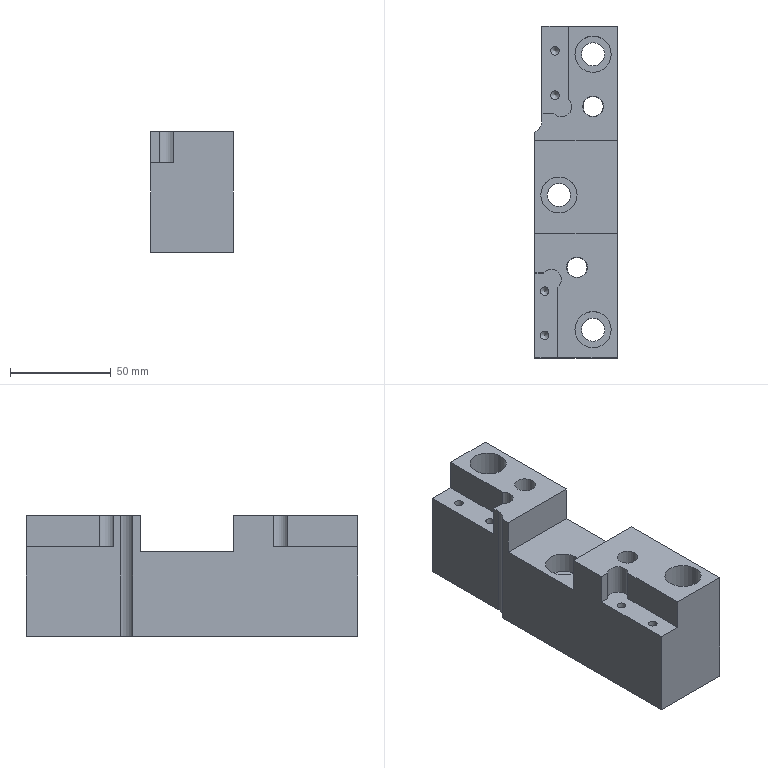Part | NX | features solid 2 | 1 solid | 43 faces | box 41 x 165 x 60 mm | volume 306635 mm3 | plane 22 | cylinder 17 | cone 4 | commonest cylinder face diameters 4.3 x4 11.5 x3 18 x3 10 x2 10.001 x2 10.3 x2
STEP:
#1=CARTESIAN_POINT('',(495.25,-4.,-30.));
#2=VERTEX_POINT('',#1);
#3=CARTESIAN_POINT('',(501.,-4.,-30.));
#4=DIRECTION('',(0.,0.,-1.));
#5=DIRECTION('',(-1.,0.,0.));
#6=AXIS2_PLACEMENT_3D('',#3,#4,#5);
#7=CIRCLE('',#6,5.75);
#8=EDGE_CURVE('',#2,#2,#7,.F.);
#9=ORIENTED_EDGE('',*,*,#8,.F.);
#10=EDGE_LOOP('',(#9));
#11=FACE_BOUND('',#10,.T.);
#12=CARTESIAN_POINT('',(492.,-4.,-30.));
#13=VERTEX_POINT('',#12);
#14=CARTESIAN_POINT('',(501.,-4.,-30.));
#15=DIRECTION('',(0.,0.,-1.));
#16=DIRECTION('',(-1.,0.,0.));
#17=AXIS2_PLACEMENT_3D('',#14,#15,#16);
#18=CIRCLE('',#17,9.);
#19=EDGE_CURVE('',#13,#13,#18,.F.);
#20=ORIENTED_EDGE('',*,*,#19,.T.);
#21=EDGE_LOOP('',(#20));
#22=FACE_BOUND('',#21,.T.);
#23=CARTESIAN_POINT('',(501.,-4.008,-30.));
#24=DIRECTION('',(0.,0.,-1.));
#25=DIRECTION('',(-1.,0.,0.));
#26=AXIS2_PLACEMENT_3D('',#23,#24,#25);
#27=PLANE('',#26);
#28=ADVANCED_FACE('',(#11,#22),#27,.F.);
#29=CARTESIAN_POINT('',(495.25,-4.,-61.5));
#30=VERTEX_POINT('',#29);
#31=CARTESIAN_POINT('',(501.,-4.,-61.5));
#32=DIRECTION('',(0.,0.,-1.));
#33=DIRECTION('',(-1.,0.,0.));
#34=AXIS2_PLACEMENT_3D('',#31,#32,#33);
#35=CIRCLE('',#34,5.75);
#36=EDGE_CURVE('',#30,#30,#35,.T.);
#37=ORIENTED_EDGE('',*,*,#36,.T.);
#38=EDGE_LOOP('',(#37));
#39=FACE_BOUND('',#38,.T.);
#40=ORIENTED_EDGE('',*,*,#8,.T.);
#41=EDGE_LOOP('',(#40));
#42=FACE_BOUND('',#41,.T.);
#43=CARTESIAN_POINT('',(501.,-4.,2.));
#44=DIRECTION('',(0.,0.,-1.));
#45=DIRECTION('',(1.,0.,0.));
#46=AXIS2_PLACEMENT_3D('',#43,#44,#45);
#47=CYLINDRICAL_SURFACE('',#46,5.75);
#48=ADVANCED_FACE('',(#39,#42),#47,.F.);
#49=CARTESIAN_POINT('',(492.,-4.,-19.5));
#50=VERTEX_POINT('',#49);
#51=CARTESIAN_POINT('',(501.,-4.,-19.5));
#52=DIRECTION('',(0.,0.,-1.));
#53=DIRECTION('',(-1.,0.,0.));
#54=AXIS2_PLACEMENT_3D('',#51,#52,#53);
#55=CIRCLE('',#54,9.);
#56=EDGE_CURVE('',#50,#50,#55,.T.);
#57=ORIENTED_EDGE('',*,*,#56,.F.);
#58=EDGE_LOOP('',(#57));
#59=FACE_BOUND('',#58,.T.);
#60=ORIENTED_EDGE('',*,*,#19,.F.);
#61=EDGE_LOOP('',(#60));
#62=FACE_BOUND('',#61,.T.);
#63=CARTESIAN_POINT('',(501.,-4.,0.));
#64=DIRECTION('',(0.,0.,-1.));
#65=DIRECTION('',(1.,0.,0.));
#66=AXIS2_PLACEMENT_3D('',#63,#64,#65);
#67=CYLINDRICAL_SURFACE('',#66,9.);
#68=ADVANCED_FACE('',(#59,#62),#67,.F.);
#69=CARTESIAN_POINT('',(498.532,36.627,-1.5));
#70=VERTEX_POINT('',#69);
#71=CARTESIAN_POINT('',(505.571,43.666,-1.5));
#72=VERTEX_POINT('',#71);
#73=CARTESIAN_POINT('',(502.389,39.809,-1.5));
#74=DIRECTION('',(0.,0.,-1.));
#75=DIRECTION('',(-1.,0.,0.));
#76=AXIS2_PLACEMENT_3D('',#73,#74,#75);
#77=CIRCLE('',#76,5.);
#78=EDGE_CURVE('',#70,#72,#77,.F.);
#79=ORIENTED_EDGE('',*,*,#78,.T.);
#80=CARTESIAN_POINT('',(505.571,43.666,-17.));
#81=VERTEX_POINT('',#80);
#82=CARTESIAN_POINT('',(505.571,43.666,-17.));
#83=DIRECTION('',(0.,0.,1.));
#84=VECTOR('',#83,1000.);
#85=LINE('',#82,#84);
#86=EDGE_CURVE('',#81,#72,#85,.T.);
#87=ORIENTED_EDGE('',*,*,#86,.F.);
#88=CARTESIAN_POINT('',(498.532,36.627,-17.));
#89=VERTEX_POINT('',#88);
#90=CARTESIAN_POINT('',(502.389,39.809,-17.));
#91=DIRECTION('',(0.,0.,1.));
#92=DIRECTION('',(1.,0.,0.));
#93=AXIS2_PLACEMENT_3D('',#90,#91,#92);
#94=CIRCLE('',#93,5.);
#95=EDGE_CURVE('',#89,#81,#94,.T.);
#96=ORIENTED_EDGE('',*,*,#95,.F.);
#97=CARTESIAN_POINT('',(498.532,36.627,-9.25));
#98=DIRECTION('',(0.,0.,1.));
#99=VECTOR('',#98,1000.);
#100=LINE('',#97,#99);
#101=EDGE_CURVE('',#70,#89,#100,.F.);
#102=ORIENTED_EDGE('',*,*,#101,.F.);
#103=EDGE_LOOP('',(#79,#87,#96,#102));
#104=FACE_BOUND('',#103,.T.);
#105=CARTESIAN_POINT('',(502.389,39.809,-17.));
#106=DIRECTION('',(0.,0.,1.));
#107=DIRECTION('',(1.,0.,0.));
#108=AXIS2_PLACEMENT_3D('',#105,#106,#107);
#109=CYLINDRICAL_SURFACE('',#108,5.);
#110=ADVANCED_FACE('',(#104),#109,.F.);
#111=CARTESIAN_POINT('',(505.571,80.,-1.5));
#112=VERTEX_POINT('',#111);
#113=CARTESIAN_POINT('',(505.571,0.,-1.5));
#114=DIRECTION('',(0.,-1.,0.));
#115=VECTOR('',#114,1000.);
#116=LINE('',#113,#115);
#117=EDGE_CURVE('',#72,#112,#116,.F.);
#118=ORIENTED_EDGE('',*,*,#117,.T.);
#119=CARTESIAN_POINT('',(505.571,80.,-17.));
#120=VERTEX_POINT('',#119);
#121=CARTESIAN_POINT('',(505.571,80.,-12.));
#122=DIRECTION('',(0.,0.,1.));
#123=VECTOR('',#122,1000.);
#124=LINE('',#121,#123);
#125=EDGE_CURVE('',#120,#112,#124,.T.);
#126=ORIENTED_EDGE('',*,*,#125,.F.);
#127=CARTESIAN_POINT('',(505.571,56.627,-17.));
#128=DIRECTION('',(0.,1.,0.));
#129=VECTOR('',#128,1000.);
#130=LINE('',#127,#129);
#131=EDGE_CURVE('',#120,#81,#130,.F.);
#132=ORIENTED_EDGE('',*,*,#131,.T.);
#133=ORIENTED_EDGE('',*,*,#86,.T.);
#134=EDGE_LOOP('',(#118,#126,#132,#133));
#135=FACE_BOUND('',#134,.T.);
#136=CARTESIAN_POINT('',(505.571,56.627,-12.));
#137=DIRECTION('',(1.,0.,0.));
#138=DIRECTION('',(0.,0.,-1.));
#139=AXIS2_PLACEMENT_3D('',#136,#137,#138);
#140=PLANE('',#139);
#141=ADVANCED_FACE('',(#135),#140,.F.);
#142=CARTESIAN_POINT('',(509.,66.,-1.5));
#143=VERTEX_POINT('',#142);
#144=CARTESIAN_POINT('',(518.,66.,-1.5));
#145=DIRECTION('',(0.,0.,-1.));
#146=DIRECTION('',(-1.,0.,0.));
#147=AXIS2_PLACEMENT_3D('',#144,#145,#146);
#148=CIRCLE('',#147,9.);
#149=EDGE_CURVE('',#143,#143,#148,.F.);
#150=ORIENTED_EDGE('',*,*,#149,.T.);
#151=EDGE_LOOP('',(#150));
#152=FACE_BOUND('',#151,.T.);
#153=CARTESIAN_POINT('',(509.,66.,-30.));
#154=VERTEX_POINT('',#153);
#155=CARTESIAN_POINT('',(518.,66.,-30.));
#156=DIRECTION('',(0.,0.,-1.));
#157=DIRECTION('',(-1.,0.,0.));
#158=AXIS2_PLACEMENT_3D('',#155,#156,#157);
#159=CIRCLE('',#158,9.);
#160=EDGE_CURVE('',#154,#154,#159,.F.);
#161=ORIENTED_EDGE('',*,*,#160,.F.);
#162=EDGE_LOOP('',(#161));
#163=FACE_BOUND('',#162,.T.);
#164=CARTESIAN_POINT('',(518.,66.,0.));
#165=DIRECTION('',(0.,0.,-1.));
#166=DIRECTION('',(1.,0.,0.));
#167=AXIS2_PLACEMENT_3D('',#164,#165,#166);
#168=CYLINDRICAL_SURFACE('',#167,9.);
#169=ADVANCED_FACE('',(#152,#163),#168,.F.);
#170=CARTESIAN_POINT('',(500.402,-85.,-1.5));
#171=VERTEX_POINT('',#170);
#172=CARTESIAN_POINT('',(500.402,-49.855,-1.5));
#173=VERTEX_POINT('',#172);
#174=CARTESIAN_POINT('',(500.402,0.,-1.5));
#175=DIRECTION('',(0.,-1.,0.));
#176=VECTOR('',#175,1000.);
#177=LINE('',#174,#176);
#178=EDGE_CURVE('',#171,#173,#177,.F.);
#179=ORIENTED_EDGE('',*,*,#178,.T.);
#180=CARTESIAN_POINT('',(500.402,-49.855,-17.));
#181=VERTEX_POINT('',#180);
#182=CARTESIAN_POINT('',(500.402,-49.855,-17.));
#183=DIRECTION('',(0.,0.,1.));
#184=VECTOR('',#183,1000.);
#185=LINE('',#182,#184);
#186=EDGE_CURVE('',#173,#181,#185,.F.);
#187=ORIENTED_EDGE('',*,*,#186,.T.);
#188=CARTESIAN_POINT('',(500.402,-85.,-17.));
#189=VERTEX_POINT('',#188);
#190=CARTESIAN_POINT('',(500.402,-62.816,-17.));
#191=DIRECTION('',(0.,-1.,0.));
#192=VECTOR('',#191,1000.);
#193=LINE('',#190,#192);
#194=EDGE_CURVE('',#181,#189,#193,.T.);
#195=ORIENTED_EDGE('',*,*,#194,.T.);
#196=CARTESIAN_POINT('',(500.402,-85.,-6.49));
#197=DIRECTION('',(0.,0.,1.));
#198=VECTOR('',#197,1000.);
#199=LINE('',#196,#198);
#200=EDGE_CURVE('',#189,#171,#199,.T.);
#201=ORIENTED_EDGE('',*,*,#200,.T.);
#202=EDGE_LOOP('',(#179,#187,#195,#201));
#203=FACE_BOUND('',#202,.T.);
#204=CARTESIAN_POINT('',(500.402,-62.816,-12.));
#205=DIRECTION('',(1.,0.,0.));
#206=DIRECTION('',(0.,0.,-1.));
#207=AXIS2_PLACEMENT_3D('',#204,#205,#206);
#208=PLANE('',#207);
#209=ADVANCED_FACE('',(#203),#208,.F.);
#210=CARTESIAN_POINT('',(493.363,-42.816,-17.));
#211=VERTEX_POINT('',#210);
#212=CARTESIAN_POINT('',(497.22,-45.998,-17.));
#213=DIRECTION('',(0.,0.,1.));
#214=DIRECTION('',(1.,0.,0.));
#215=AXIS2_PLACEMENT_3D('',#212,#213,#214);
#216=CIRCLE('',#215,5.);
#217=EDGE_CURVE('',#181,#211,#216,.T.);
#218=ORIENTED_EDGE('',*,*,#217,.F.);
#219=ORIENTED_EDGE('',*,*,#186,.F.);
#220=CARTESIAN_POINT('',(493.363,-42.816,-1.5));
#221=VERTEX_POINT('',#220);
#222=CARTESIAN_POINT('',(497.22,-45.998,-1.5));
#223=DIRECTION('',(0.,0.,-1.));
#224=DIRECTION('',(-1.,0.,0.));
#225=AXIS2_PLACEMENT_3D('',#222,#223,#224);
#226=CIRCLE('',#225,5.);
#227=EDGE_CURVE('',#173,#221,#226,.F.);
#228=ORIENTED_EDGE('',*,*,#227,.T.);
#229=CARTESIAN_POINT('',(493.363,-42.816,-9.25));
#230=DIRECTION('',(0.,0.,1.));
#231=VECTOR('',#230,1000.);
#232=LINE('',#229,#231);
#233=EDGE_CURVE('',#211,#221,#232,.T.);
#234=ORIENTED_EDGE('',*,*,#233,.F.);
#235=EDGE_LOOP('',(#218,#219,#228,#234));
#236=FACE_BOUND('',#235,.T.);
#237=CARTESIAN_POINT('',(497.22,-45.998,-17.));
#238=DIRECTION('',(0.,0.,1.));
#239=DIRECTION('',(1.,0.,0.));
#240=AXIS2_PLACEMENT_3D('',#237,#238,#239);
#241=CYLINDRICAL_SURFACE('',#240,5.);
#242=ADVANCED_FACE('',(#236),#241,.F.);
#243=CARTESIAN_POINT('',(509.,-71.,-1.5));
#244=VERTEX_POINT('',#243);
#245=CARTESIAN_POINT('',(518.,-71.,-1.5));
#246=DIRECTION('',(0.,0.,-1.));
#247=DIRECTION('',(-1.,0.,0.));
#248=AXIS2_PLACEMENT_3D('',#245,#246,#247);
#249=CIRCLE('',#248,9.);
#250=EDGE_CURVE('',#244,#244,#249,.F.);
#251=ORIENTED_EDGE('',*,*,#250,.T.);
#252=EDGE_LOOP('',(#251));
#253=FACE_BOUND('',#252,.T.);
#254=CARTESIAN_POINT('',(509.,-71.,-30.));
#255=VERTEX_POINT('',#254);
#256=CARTESIAN_POINT('',(518.,-71.,-30.));
#257=DIRECTION('',(0.,0.,-1.));
#258=DIRECTION('',(-1.,0.,0.));
#259=AXIS2_PLACEMENT_3D('',#256,#257,#258);
#260=CIRCLE('',#259,9.);
#261=EDGE_CURVE('',#255,#255,#260,.F.);
#262=ORIENTED_EDGE('',*,*,#261,.F.);
#263=EDGE_LOOP('',(#262));
#264=FACE_BOUND('',#263,.T.);
#265=CARTESIAN_POINT('',(518.,-71.,0.));
#266=DIRECTION('',(0.,0.,-1.));
#267=DIRECTION('',(1.,0.,0.));
#268=AXIS2_PLACEMENT_3D('',#265,#266,#267);
#269=CYLINDRICAL_SURFACE('',#268,9.);
#270=ADVANCED_FACE('',(#253,#264),#269,.F.);
#271=CARTESIAN_POINT('',(492.571,36.627,-1.5));
#272=VERTEX_POINT('',#271);
#273=CARTESIAN_POINT('',(386.,36.627,-1.5));
#274=DIRECTION('',(-1.,0.,0.));
#275=VECTOR('',#274,1000.);
#276=LINE('',#273,#275);
#277=EDGE_CURVE('',#272,#70,#276,.F.);
#278=ORIENTED_EDGE('',*,*,#277,.T.);
#279=ORIENTED_EDGE('',*,*,#101,.T.);
#280=CARTESIAN_POINT('',(492.571,36.627,-17.));
#281=VERTEX_POINT('',#280);
#282=CARTESIAN_POINT('',(495.571,36.627,-17.));
#283=DIRECTION('',(-1.,0.,0.));
#284=VECTOR('',#283,1000.);
#285=LINE('',#282,#284);
#286=EDGE_CURVE('',#89,#281,#285,.T.);
#287=ORIENTED_EDGE('',*,*,#286,.T.);
#288=CARTESIAN_POINT('',(492.571,36.627,-89.727));
#289=DIRECTION('',(0.,0.,1.));
#290=VECTOR('',#289,1000.);
#291=LINE('',#288,#290);
#292=EDGE_CURVE('',#281,#272,#291,.T.);
#293=ORIENTED_EDGE('',*,*,#292,.T.);
#294=EDGE_LOOP('',(#278,#279,#287,#293));
#295=FACE_BOUND('',#294,.T.);
#296=CARTESIAN_POINT('',(495.571,36.627,-12.));
#297=DIRECTION('',(0.,-1.,0.));
#298=DIRECTION('',(0.,0.,-1.));
#299=AXIS2_PLACEMENT_3D('',#296,#297,#298);
#300=PLANE('',#299);
#301=ADVANCED_FACE('',(#295),#300,.F.);
#302=CARTESIAN_POINT('',(501.221,45.627,-17.));
#303=VERTEX_POINT('',#302);
#304=CARTESIAN_POINT('',(499.071,45.627,-17.));
#305=DIRECTION('',(0.,0.,-1.));
#306=DIRECTION('',(1.,0.,0.));
#307=AXIS2_PLACEMENT_3D('',#304,#305,#306);
#308=CIRCLE('',#307,2.15);
#309=EDGE_CURVE('',#303,#303,#308,.T.);
#310=ORIENTED_EDGE('',*,*,#309,.T.);
#311=EDGE_LOOP('',(#310));
#312=FACE_BOUND('',#311,.T.);
#313=CARTESIAN_POINT('',(501.221,67.627,-17.));
#314=VERTEX_POINT('',#313);
#315=CARTESIAN_POINT('',(499.071,67.627,-17.));
#316=DIRECTION('',(0.,0.,-1.));
#317=DIRECTION('',(1.,0.,0.));
#318=AXIS2_PLACEMENT_3D('',#315,#316,#317);
#319=CIRCLE('',#318,2.15);
#320=EDGE_CURVE('',#314,#314,#319,.T.);
#321=ORIENTED_EDGE('',*,*,#320,.T.);
#322=EDGE_LOOP('',(#321));
#323=FACE_BOUND('',#322,.T.);
#324=ORIENTED_EDGE('',*,*,#131,.F.);
#325=CARTESIAN_POINT('',(492.571,80.,-17.));
#326=VERTEX_POINT('',#325);
#327=CARTESIAN_POINT('',(495.571,80.,-17.));
#328=DIRECTION('',(1.,0.,0.));
#329=VECTOR('',#328,1000.);
#330=LINE('',#327,#329);
#331=EDGE_CURVE('',#326,#120,#330,.T.);
#332=ORIENTED_EDGE('',*,*,#331,.F.);
#333=CARTESIAN_POINT('',(492.571,56.627,-17.));
#334=DIRECTION('',(0.,-1.,0.));
#335=VECTOR('',#334,1000.);
#336=LINE('',#333,#335);
#337=EDGE_CURVE('',#281,#326,#336,.F.);
#338=ORIENTED_EDGE('',*,*,#337,.F.);
#339=ORIENTED_EDGE('',*,*,#286,.F.);
#340=ORIENTED_EDGE('',*,*,#95,.T.);
#341=EDGE_LOOP('',(#324,#332,#338,#339,#340));
#342=FACE_BOUND('',#341,.T.);
#343=CARTESIAN_POINT('',(495.571,56.627,-17.));
#344=DIRECTION('',(0.,0.,-1.));
#345=DIRECTION('',(-1.,0.,0.));
#346=AXIS2_PLACEMENT_3D('',#343,#344,#345);
#347=PLANE('',#346);
#348=ADVANCED_FACE('',(#312,#323,#342),#347,.F.);
#349=CARTESIAN_POINT('',(489.,-42.816,-17.));
#350=VERTEX_POINT('',#349);
#351=CARTESIAN_POINT('',(489.,-42.816,-1.5));
#352=VERTEX_POINT('',#351);
#353=CARTESIAN_POINT('',(489.,-42.816,-12.));
#354=DIRECTION('',(0.,0.,1.));
#355=VECTOR('',#354,1000.);
#356=LINE('',#353,#355);
#357=EDGE_CURVE('',#350,#352,#356,.T.);
#358=ORIENTED_EDGE('',*,*,#357,.F.);
#359=CARTESIAN_POINT('',(490.402,-42.816,-17.));
#360=DIRECTION('',(1.,0.,0.));
#361=VECTOR('',#360,1000.);
#362=LINE('',#359,#361);
#363=EDGE_CURVE('',#350,#211,#362,.T.);
#364=ORIENTED_EDGE('',*,*,#363,.T.);
#365=ORIENTED_EDGE('',*,*,#233,.T.);
#366=CARTESIAN_POINT('',(386.,-42.816,-1.5));
#367=DIRECTION('',(1.,0.,0.));
#368=VECTOR('',#367,1000.);
#369=LINE('',#366,#368);
#370=EDGE_CURVE('',#221,#352,#369,.F.);
#371=ORIENTED_EDGE('',*,*,#370,.T.);
#372=EDGE_LOOP('',(#358,#364,#365,#371));
#373=FACE_BOUND('',#372,.T.);
#374=CARTESIAN_POINT('',(490.402,-42.816,-12.));
#375=DIRECTION('',(0.,1.,0.));
#376=DIRECTION('',(0.,0.,1.));
#377=AXIS2_PLACEMENT_3D('',#374,#375,#376);
#378=PLANE('',#377);
#379=ADVANCED_FACE('',(#373),#378,.F.);
#380=CARTESIAN_POINT('',(496.052,-73.816,-17.));
#381=VERTEX_POINT('',#380);
#382=CARTESIAN_POINT('',(493.902,-73.816,-17.));
#383=DIRECTION('',(0.,0.,-1.));
#384=DIRECTION('',(1.,0.,0.));
#385=AXIS2_PLACEMENT_3D('',#382,#383,#384);
#386=CIRCLE('',#385,2.15);
#387=EDGE_CURVE('',#381,#381,#386,.T.);
#388=ORIENTED_EDGE('',*,*,#387,.T.);
#389=EDGE_LOOP('',(#388));
#390=FACE_BOUND('',#389,.T.);
#391=CARTESIAN_POINT('',(496.052,-51.816,-17.));
#392=VERTEX_POINT('',#391);
#393=CARTESIAN_POINT('',(493.902,-51.816,-17.));
#394=DIRECTION('',(0.,0.,-1.));
#395=DIRECTION('',(1.,0.,0.));
#396=AXIS2_PLACEMENT_3D('',#393,#394,#395);
#397=CIRCLE('',#396,2.15);
#398=EDGE_CURVE('',#392,#392,#397,.T.);
#399=ORIENTED_EDGE('',*,*,#398,.T.);
#400=EDGE_LOOP('',(#399));
#401=FACE_BOUND('',#400,.T.);
#402=CARTESIAN_POINT('',(489.,-85.,-17.));
#403=VERTEX_POINT('',#402);
#404=CARTESIAN_POINT('',(489.,-62.816,-17.));
#405=DIRECTION('',(0.,1.,0.));
#406=VECTOR('',#405,1000.);
#407=LINE('',#404,#406);
#408=EDGE_CURVE('',#403,#350,#407,.T.);
#409=ORIENTED_EDGE('',*,*,#408,.F.);
#410=CARTESIAN_POINT('',(490.402,-85.,-17.));
#411=DIRECTION('',(-1.,0.,0.));
#412=VECTOR('',#411,1000.);
#413=LINE('',#410,#412);
#414=EDGE_CURVE('',#189,#403,#413,.T.);
#415=ORIENTED_EDGE('',*,*,#414,.F.);
#416=ORIENTED_EDGE('',*,*,#194,.F.);
#417=ORIENTED_EDGE('',*,*,#217,.T.);
#418=ORIENTED_EDGE('',*,*,#363,.F.);
#419=EDGE_LOOP('',(#409,#415,#416,#417,#418));
#420=FACE_BOUND('',#419,.T.);
#421=CARTESIAN_POINT('',(490.402,-62.816,-17.));
#422=DIRECTION('',(0.,0.,-1.));
#423=DIRECTION('',(-1.,0.,0.));
#424=AXIS2_PLACEMENT_3D('',#421,#422,#423);
#425=PLANE('',#424);
#426=ADVANCED_FACE('',(#390,#401,#420),#425,.F.);
#427=CARTESIAN_POINT('',(512.25,-71.,-30.));
#428=VERTEX_POINT('',#427);
#429=CARTESIAN_POINT('',(518.,-71.,-30.));
#430=DIRECTION('',(0.,0.,-1.));
#431=DIRECTION('',(-1.,0.,0.));
#432=AXIS2_PLACEMENT_3D('',#429,#430,#431);
#433=CIRCLE('',#432,5.75);
#434=EDGE_CURVE('',#428,#428,#433,.F.);
#435=ORIENTED_EDGE('',*,*,#434,.F.);
#436=EDGE_LOOP('',(#435));
#437=FACE_BOUND('',#436,.T.);
#438=ORIENTED_EDGE('',*,*,#261,.T.);
#439=EDGE_LOOP('',(#438));
#440=FACE_BOUND('',#439,.T.);
#441=CARTESIAN_POINT('',(518.,-71.008,-30.));
#442=DIRECTION('',(0.,0.,-1.));
#443=DIRECTION('',(-1.,0.,0.));
#444=AXIS2_PLACEMENT_3D('',#441,#442,#443);
#445=PLANE('',#444);
#446=ADVANCED_FACE('',(#437,#440),#445,.F.);
#447=CARTESIAN_POINT('',(512.25,66.,-30.));
#448=VERTEX_POINT('',#447);
#449=CARTESIAN_POINT('',(518.,66.,-30.));
#450=DIRECTION('',(0.,0.,-1.));
#451=DIRECTION('',(-1.,0.,0.));
#452=AXIS2_PLACEMENT_3D('',#449,#450,#451);
#453=CIRCLE('',#452,5.75);
#454=EDGE_CURVE('',#448,#448,#453,.F.);
#455=ORIENTED_EDGE('',*,*,#454,.F.);
#456=EDGE_LOOP('',(#455));
#457=FACE_BOUND('',#456,.T.);
#458=ORIENTED_EDGE('',*,*,#160,.T.);
#459=EDGE_LOOP('',(#458));
#460=FACE_BOUND('',#459,.T.);
#461=CARTESIAN_POINT('',(518.,66.017,-30.));
#462=DIRECTION('',(0.,0.,-1.));
#463=DIRECTION('',(-1.,0.,0.));
#464=AXIS2_PLACEMENT_3D('',#461,#462,#463);
#465=PLANE('',#464);
#466=ADVANCED_FACE('',(#457,#460),#465,.F.);
#467=CARTESIAN_POINT('',(512.85,40.,-1.5));
#468=VERTEX_POINT('',#467);
#469=CARTESIAN_POINT('',(518.,40.,-1.5));
#470=DIRECTION('',(0.,0.,-1.));
#471=DIRECTION('',(-1.,0.,0.));
#472=AXIS2_PLACEMENT_3D('',#469,#470,#471);
#473=CIRCLE('',#472,5.15);
#474=EDGE_CURVE('',#468,#468,#473,.T.);
#475=ORIENTED_EDGE('',*,*,#474,.T.);
#476=EDGE_LOOP('',(#475));
#477=FACE_BOUND('',#476,.T.);
#478=CARTESIAN_POINT('',(530.,80.,-1.5));
#479=VERTEX_POINT('',#478);
#480=CARTESIAN_POINT('',(419.237,80.,-1.5));
#481=DIRECTION('',(-1.,0.,0.));
#482=VECTOR('',#481,1000.);
#483=LINE('',#480,#482);
#484=EDGE_CURVE('',#112,#479,#483,.F.);
#485=ORIENTED_EDGE('',*,*,#484,.F.);
#486=ORIENTED_EDGE('',*,*,#117,.F.);
#487=ORIENTED_EDGE('',*,*,#78,.F.);
#488=ORIENTED_EDGE('',*,*,#277,.F.);
#489=CARTESIAN_POINT('',(492.571,33.127,-1.5));
#490=VERTEX_POINT('',#489);
#491=CARTESIAN_POINT('',(492.571,78.127,-1.5));
#492=DIRECTION('',(0.,-1.,0.));
#493=VECTOR('',#492,1000.);
#494=LINE('',#491,#493);
#495=EDGE_CURVE('',#490,#272,#494,.F.);
#496=ORIENTED_EDGE('',*,*,#495,.F.);
#497=CARTESIAN_POINT('',(489.,27.025,-1.5));
#498=VERTEX_POINT('',#497);
#499=CARTESIAN_POINT('',(485.571,33.127,-1.5));
#500=DIRECTION('',(0.,0.,-1.));
#501=DIRECTION('',(-1.,0.,0.));
#502=AXIS2_PLACEMENT_3D('',#499,#500,#501);
#503=CIRCLE('',#502,7.);
#504=EDGE_CURVE('',#498,#490,#503,.F.);
#505=ORIENTED_EDGE('',*,*,#504,.F.);
#506=CARTESIAN_POINT('',(489.,23.,-1.5));
#507=VERTEX_POINT('',#506);
#508=CARTESIAN_POINT('',(489.,0.,-1.5));
#509=DIRECTION('',(0.,1.,0.));
#510=VECTOR('',#509,1000.);
#511=LINE('',#508,#510);
#512=EDGE_CURVE('',#498,#507,#511,.F.);
#513=ORIENTED_EDGE('',*,*,#512,.T.);
#514=CARTESIAN_POINT('',(530.,23.,-1.5));
#515=VERTEX_POINT('',#514);
#516=CARTESIAN_POINT('',(386.,23.,-1.5));
#517=DIRECTION('',(1.,0.,0.));
#518=VECTOR('',#517,1000.);
#519=LINE('',#516,#518);
#520=EDGE_CURVE('',#515,#507,#519,.F.);
#521=ORIENTED_EDGE('',*,*,#520,.F.);
#522=CARTESIAN_POINT('',(530.,108.,-1.5));
#523=DIRECTION('',(0.,1.,0.));
#524=VECTOR('',#523,1000.);
#525=LINE('',#522,#524);
#526=EDGE_CURVE('',#479,#515,#525,.F.);
#527=ORIENTED_EDGE('',*,*,#526,.F.);
#528=EDGE_LOOP('',(#485,#486,#487,#488,#496,#505,#513,#521,#527));
#529=FACE_BOUND('',#528,.T.);
#530=ORIENTED_EDGE('',*,*,#149,.F.);
#531=EDGE_LOOP('',(#530));
#532=FACE_BOUND('',#531,.T.);
#533=CARTESIAN_POINT('',(386.,0.,-1.5));
#534=DIRECTION('',(0.,0.,-1.));
#535=DIRECTION('',(-1.,0.,0.));
#536=AXIS2_PLACEMENT_3D('',#533,#534,#535);
#537=PLANE('',#536);
#538=ADVANCED_FACE('',(#477,#529,#532),#537,.F.);
#539=CARTESIAN_POINT('',(504.85,-40.,-1.5));
#540=VERTEX_POINT('',#539);
#541=CARTESIAN_POINT('',(510.,-40.,-1.5));
#542=DIRECTION('',(0.,0.,-1.));
#543=DIRECTION('',(-1.,0.,0.));
#544=AXIS2_PLACEMENT_3D('',#541,#542,#543);
#545=CIRCLE('',#544,5.15);
#546=EDGE_CURVE('',#540,#540,#545,.T.);
#547=ORIENTED_EDGE('',*,*,#546,.T.);
#548=EDGE_LOOP('',(#547));
#549=FACE_BOUND('',#548,.T.);
#550=ORIENTED_EDGE('',*,*,#250,.F.);
#551=EDGE_LOOP('',(#550));
#552=FACE_BOUND('',#551,.T.);
#553=CARTESIAN_POINT('',(530.,-23.,-1.5));
#554=VERTEX_POINT('',#553);
#555=CARTESIAN_POINT('',(530.,-85.,-1.5));
#556=VERTEX_POINT('',#555);
#557=CARTESIAN_POINT('',(530.,108.,-1.5));
#558=DIRECTION('',(0.,1.,0.));
#559=VECTOR('',#558,1000.);
#560=LINE('',#557,#559);
#561=EDGE_CURVE('',#554,#556,#560,.F.);
#562=ORIENTED_EDGE('',*,*,#561,.F.);
#563=CARTESIAN_POINT('',(489.,-23.,-1.5));
#564=VERTEX_POINT('',#563);
#565=CARTESIAN_POINT('',(386.,-23.,-1.5));
#566=DIRECTION('',(-1.,0.,0.));
#567=VECTOR('',#566,1000.);
#568=LINE('',#565,#567);
#569=EDGE_CURVE('',#564,#554,#568,.F.);
#570=ORIENTED_EDGE('',*,*,#569,.F.);
#571=CARTESIAN_POINT('',(489.,0.,-1.5));
#572=DIRECTION('',(0.,1.,0.));
#573=VECTOR('',#572,1000.);
#574=LINE('',#571,#573);
#575=EDGE_CURVE('',#564,#352,#574,.F.);
#576=ORIENTED_EDGE('',*,*,#575,.T.);
#577=ORIENTED_EDGE('',*,*,#370,.F.);
#578=ORIENTED_EDGE('',*,*,#227,.F.);
#579=ORIENTED_EDGE('',*,*,#178,.F.);
#580=CARTESIAN_POINT('',(386.,-85.,-1.5));
#581=DIRECTION('',(-1.,0.,0.));
#582=VECTOR('',#581,1000.);
#583=LINE('',#580,#582);
#584=EDGE_CURVE('',#171,#556,#583,.F.);
#585=ORIENTED_EDGE('',*,*,#584,.T.);
#586=EDGE_LOOP('',(#562,#570,#576,#577,#578,#579,#585));
#587=FACE_BOUND('',#586,.T.);
#588=CARTESIAN_POINT('',(386.,0.,-1.5));
#589=DIRECTION('',(0.,0.,-1.));
#590=DIRECTION('',(-1.,0.,0.));
#591=AXIS2_PLACEMENT_3D('',#588,#589,#590);
#592=PLANE('',#591);
#593=ADVANCED_FACE('',(#549,#552,#587),#592,.F.);
#594=CARTESIAN_POINT('',(530.,-23.,-19.5));
#595=VERTEX_POINT('',#594);
#596=CARTESIAN_POINT('',(530.,-23.,0.));
#597=DIRECTION('',(0.,0.,-1.));
#598=VECTOR('',#597,1000.);
#599=LINE('',#596,#598);
#600=EDGE_CURVE('',#554,#595,#599,.T.);
#601=ORIENTED_EDGE('',*,*,#600,.T.);
#602=CARTESIAN_POINT('',(489.,-23.,-19.5));
#603=VERTEX_POINT('',#602);
#604=CARTESIAN_POINT('',(386.,-23.,-19.5));
#605=DIRECTION('',(-1.,0.,0.));
#606=VECTOR('',#605,1000.);
#607=LINE('',#604,#606);
#608=EDGE_CURVE('',#595,#603,#607,.T.);
#609=ORIENTED_EDGE('',*,*,#608,.T.);
#610=CARTESIAN_POINT('',(489.,-23.,-19.));
#611=DIRECTION('',(0.,0.,1.));
#612=VECTOR('',#611,1000.);
#613=LINE('',#610,#612);
#614=EDGE_CURVE('',#603,#564,#613,.T.);
#615=ORIENTED_EDGE('',*,*,#614,.T.);
#616=ORIENTED_EDGE('',*,*,#569,.T.);
#617=EDGE_LOOP('',(#601,#609,#615,#616));
#618=FACE_BOUND('',#617,.T.);
#619=CARTESIAN_POINT('',(365.,-23.,-51.5));
#620=DIRECTION('',(0.,-1.,0.));
#621=DIRECTION('',(0.,0.,-1.));
#622=AXIS2_PLACEMENT_3D('',#619,#620,#621);
#623=PLANE('',#622);
#624=ADVANCED_FACE('',(#618),#623,.F.);
#625=CARTESIAN_POINT('',(530.,23.,-19.5));
#626=VERTEX_POINT('',#625);
#627=CARTESIAN_POINT('',(530.,23.,0.));
#628=DIRECTION('',(0.,0.,1.));
#629=VECTOR('',#628,1000.);
#630=LINE('',#627,#629);
#631=EDGE_CURVE('',#626,#515,#630,.T.);
#632=ORIENTED_EDGE('',*,*,#631,.T.);
#633=ORIENTED_EDGE('',*,*,#520,.T.);
#634=CARTESIAN_POINT('',(489.,23.,-19.5));
#635=VERTEX_POINT('',#634);
#636=CARTESIAN_POINT('',(489.,23.,-19.));
#637=DIRECTION('',(0.,0.,-1.));
#638=VECTOR('',#637,1000.);
#639=LINE('',#636,#638);
#640=EDGE_CURVE('',#507,#635,#639,.T.);
#641=ORIENTED_EDGE('',*,*,#640,.T.);
#642=CARTESIAN_POINT('',(386.,23.,-19.5));
#643=DIRECTION('',(1.,0.,0.));
#644=VECTOR('',#643,1000.);
#645=LINE('',#642,#644);
#646=EDGE_CURVE('',#635,#626,#645,.T.);
#647=ORIENTED_EDGE('',*,*,#646,.T.);
#648=EDGE_LOOP('',(#632,#633,#641,#647));
#649=FACE_BOUND('',#648,.T.);
#650=CARTESIAN_POINT('',(365.,23.,-51.5));
#651=DIRECTION('',(0.,1.,0.));
#652=DIRECTION('',(0.,0.,1.));
#653=AXIS2_PLACEMENT_3D('',#650,#651,#652);
#654=PLANE('',#653);
#655=ADVANCED_FACE('',(#649),#654,.F.);
#656=ORIENTED_EDGE('',*,*,#526,.T.);
#657=ORIENTED_EDGE('',*,*,#631,.F.);
#658=CARTESIAN_POINT('',(530.,108.,-19.5));
#659=DIRECTION('',(0.,1.,0.));
#660=VECTOR('',#659,1000.);
#661=LINE('',#658,#660);
#662=EDGE_CURVE('',#595,#626,#661,.T.);
#663=ORIENTED_EDGE('',*,*,#662,.F.);
#664=ORIENTED_EDGE('',*,*,#600,.F.);
#665=ORIENTED_EDGE('',*,*,#561,.T.);
#666=CARTESIAN_POINT('',(530.,-85.,-61.5));
#667=VERTEX_POINT('',#666);
#668=CARTESIAN_POINT('',(530.,-85.,-6.49));
#669=DIRECTION('',(0.,0.,1.));
#670=VECTOR('',#669,1000.);
#671=LINE('',#668,#670);
#672=EDGE_CURVE('',#667,#556,#671,.T.);
#673=ORIENTED_EDGE('',*,*,#672,.F.);
#674=CARTESIAN_POINT('',(530.,80.,-61.5));
#675=VERTEX_POINT('',#674);
#676=CARTESIAN_POINT('',(530.,108.,-61.5));
#677=DIRECTION('',(0.,1.,0.));
#678=VECTOR('',#677,1000.);
#679=LINE('',#676,#678);
#680=EDGE_CURVE('',#667,#675,#679,.T.);
#681=ORIENTED_EDGE('',*,*,#680,.T.);
#682=CARTESIAN_POINT('',(530.,80.,0.));
#683=DIRECTION('',(0.,0.,1.));
#684=VECTOR('',#683,1000.);
#685=LINE('',#682,#684);
#686=EDGE_CURVE('',#675,#479,#685,.T.);
#687=ORIENTED_EDGE('',*,*,#686,.T.);
#688=EDGE_LOOP('',(#656,#657,#663,#664,#665,#673,#681,#687));
#689=FACE_BOUND('',#688,.T.);
#690=CARTESIAN_POINT('',(530.,108.,0.));
#691=DIRECTION('',(1.,0.,0.));
#692=DIRECTION('',(0.,0.,-1.));
#693=AXIS2_PLACEMENT_3D('',#690,#691,#692);
#694=PLANE('',#693);
#695=ADVANCED_FACE('',(#689),#694,.T.);
#696=ORIENTED_EDGE('',*,*,#331,.T.);
#697=ORIENTED_EDGE('',*,*,#125,.T.);
#698=ORIENTED_EDGE('',*,*,#484,.T.);
#699=ORIENTED_EDGE('',*,*,#686,.F.);
#700=CARTESIAN_POINT('',(492.571,80.,-61.5));
#701=VERTEX_POINT('',#700);
#702=CARTESIAN_POINT('',(419.237,80.,-61.5));
#703=DIRECTION('',(-1.,0.,0.));
#704=VECTOR('',#703,1000.);
#705=LINE('',#702,#704);
#706=EDGE_CURVE('',#675,#701,#705,.T.);
#707=ORIENTED_EDGE('',*,*,#706,.T.);
#708=CARTESIAN_POINT('',(492.571,80.,-89.727));
#709=DIRECTION('',(0.,0.,-1.));
#710=VECTOR('',#709,1000.);
#711=LINE('',#708,#710);
#712=EDGE_CURVE('',#326,#701,#711,.T.);
#713=ORIENTED_EDGE('',*,*,#712,.F.);
#714=EDGE_LOOP('',(#696,#697,#698,#699,#707,#713));
#715=FACE_BOUND('',#714,.T.);
#716=CARTESIAN_POINT('',(419.237,80.,-6.49));
#717=DIRECTION('',(0.,1.,0.));
#718=DIRECTION('',(0.,0.,1.));
#719=AXIS2_PLACEMENT_3D('',#716,#717,#718);
#720=PLANE('',#719);
#721=ADVANCED_FACE('',(#715),#720,.T.);
#722=ORIENTED_EDGE('',*,*,#337,.T.);
#723=ORIENTED_EDGE('',*,*,#712,.T.);
#724=CARTESIAN_POINT('',(492.571,33.127,-61.5));
#725=VERTEX_POINT('',#724);
#726=CARTESIAN_POINT('',(492.571,78.127,-61.5));
#727=DIRECTION('',(0.,-1.,0.));
#728=VECTOR('',#727,1000.);
#729=LINE('',#726,#728);
#730=EDGE_CURVE('',#701,#725,#729,.T.);
#731=ORIENTED_EDGE('',*,*,#730,.T.);
#732=CARTESIAN_POINT('',(492.571,33.127,-20.745));
#733=DIRECTION('',(0.,0.,-1.));
#734=VECTOR('',#733,1000.);
#735=LINE('',#732,#734);
#736=EDGE_CURVE('',#725,#490,#735,.F.);
#737=ORIENTED_EDGE('',*,*,#736,.T.);
#738=ORIENTED_EDGE('',*,*,#495,.T.);
#739=ORIENTED_EDGE('',*,*,#292,.F.);
#740=EDGE_LOOP('',(#722,#723,#731,#737,#738,#739));
#741=FACE_BOUND('',#740,.T.);
#742=CARTESIAN_POINT('',(492.571,78.127,-89.727));
#743=DIRECTION('',(-1.,0.,0.));
#744=DIRECTION('',(0.,0.,1.));
#745=AXIS2_PLACEMENT_3D('',#742,#743,#744);
#746=PLANE('',#745);
#747=ADVANCED_FACE('',(#741),#746,.T.);
#748=CARTESIAN_POINT('',(489.,27.025,-61.5));
#749=VERTEX_POINT('',#748);
#750=CARTESIAN_POINT('',(485.571,33.127,-61.5));
#751=DIRECTION('',(0.,0.,-1.));
#752=DIRECTION('',(-1.,0.,0.));
#753=AXIS2_PLACEMENT_3D('',#750,#751,#752);
#754=CIRCLE('',#753,7.);
#755=EDGE_CURVE('',#725,#749,#754,.T.);
#756=ORIENTED_EDGE('',*,*,#755,.T.);
#757=CARTESIAN_POINT('',(489.,27.025,-89.727));
#758=DIRECTION('',(0.,0.,-1.));
#759=VECTOR('',#758,1000.);
#760=LINE('',#757,#759);
#761=EDGE_CURVE('',#749,#498,#760,.F.);
#762=ORIENTED_EDGE('',*,*,#761,.T.);
#763=ORIENTED_EDGE('',*,*,#504,.T.);
#764=ORIENTED_EDGE('',*,*,#736,.F.);
#765=EDGE_LOOP('',(#756,#762,#763,#764));
#766=FACE_BOUND('',#765,.T.);
#767=CARTESIAN_POINT('',(485.571,33.127,-89.727));
#768=DIRECTION('',(0.,0.,-1.));
#769=DIRECTION('',(-1.,0.,0.));
#770=AXIS2_PLACEMENT_3D('',#767,#768,#769);
#771=CYLINDRICAL_SURFACE('',#770,7.);
#772=ADVANCED_FACE('',(#766),#771,.F.);
#773=ORIENTED_EDGE('',*,*,#575,.F.);
#774=ORIENTED_EDGE('',*,*,#614,.F.);
#775=CARTESIAN_POINT('',(489.,0.,-19.5));
#776=DIRECTION('',(0.,-1.,0.));
#777=VECTOR('',#776,1000.);
#778=LINE('',#775,#777);
#779=EDGE_CURVE('',#635,#603,#778,.T.);
#780=ORIENTED_EDGE('',*,*,#779,.F.);
#781=ORIENTED_EDGE('',*,*,#640,.F.);
#782=ORIENTED_EDGE('',*,*,#512,.F.);
#783=ORIENTED_EDGE('',*,*,#761,.F.);
#784=CARTESIAN_POINT('',(489.,-85.,-61.5));
#785=VERTEX_POINT('',#784);
#786=CARTESIAN_POINT('',(489.,0.,-61.5));
#787=DIRECTION('',(0.,1.,0.));
#788=VECTOR('',#787,1000.);
#789=LINE('',#786,#788);
#790=EDGE_CURVE('',#785,#749,#789,.T.);
#791=ORIENTED_EDGE('',*,*,#790,.F.);
#792=CARTESIAN_POINT('',(489.,-85.,-6.49));
#793=DIRECTION('',(0.,0.,-1.));
#794=VECTOR('',#793,1000.);
#795=LINE('',#792,#794);
#796=EDGE_CURVE('',#403,#785,#795,.T.);
#797=ORIENTED_EDGE('',*,*,#796,.F.);
#798=ORIENTED_EDGE('',*,*,#408,.T.);
#799=ORIENTED_EDGE('',*,*,#357,.T.);
#800=EDGE_LOOP('',(#773,#774,#780,#781,#782,#783,#791,#797,#798,#799));
#801=FACE_BOUND('',#800,.T.);
#802=CARTESIAN_POINT('',(489.,0.,-19.));
#803=DIRECTION('',(-1.,0.,0.));
#804=DIRECTION('',(0.,0.,1.));
#805=AXIS2_PLACEMENT_3D('',#802,#803,#804);
#806=PLANE('',#805);
#807=ADVANCED_FACE('',(#801),#806,.T.);
#808=ORIENTED_EDGE('',*,*,#200,.F.);
#809=ORIENTED_EDGE('',*,*,#414,.T.);
#810=ORIENTED_EDGE('',*,*,#796,.T.);
#811=CARTESIAN_POINT('',(419.237,-85.,-61.5));
#812=DIRECTION('',(1.,0.,0.));
#813=VECTOR('',#812,1000.);
#814=LINE('',#811,#813);
#815=EDGE_CURVE('',#785,#667,#814,.T.);
#816=ORIENTED_EDGE('',*,*,#815,.T.);
#817=ORIENTED_EDGE('',*,*,#672,.T.);
#818=ORIENTED_EDGE('',*,*,#584,.F.);
#819=EDGE_LOOP('',(#808,#809,#810,#816,#817,#818));
#820=FACE_BOUND('',#819,.T.);
#821=CARTESIAN_POINT('',(419.237,-85.,-6.49));
#822=DIRECTION('',(0.,-1.,0.));
#823=DIRECTION('',(0.,0.,-1.));
#824=AXIS2_PLACEMENT_3D('',#821,#822,#823);
#825=PLANE('',#824);
#826=ADVANCED_FACE('',(#820),#825,.T.);
#827=CARTESIAN_POINT('',(512.25,-71.,-61.5));
#828=VERTEX_POINT('',#827);
#829=CARTESIAN_POINT('',(518.,-71.,-61.5));
#830=DIRECTION('',(0.,0.,-1.));
#831=DIRECTION('',(-1.,0.,0.));
#832=AXIS2_PLACEMENT_3D('',#829,#830,#831);
#833=CIRCLE('',#832,5.75);
#834=EDGE_CURVE('',#828,#828,#833,.T.);
#835=ORIENTED_EDGE('',*,*,#834,.T.);
#836=EDGE_LOOP('',(#835));
#837=FACE_BOUND('',#836,.T.);
#838=ORIENTED_EDGE('',*,*,#434,.T.);
#839=EDGE_LOOP('',(#838));
#840=FACE_BOUND('',#839,.T.);
#841=CARTESIAN_POINT('',(518.,-71.,2.));
#842=DIRECTION('',(0.,0.,-1.));
#843=DIRECTION('',(1.,0.,0.));
#844=AXIS2_PLACEMENT_3D('',#841,#842,#843);
#845=CYLINDRICAL_SURFACE('',#844,5.75);
#846=ADVANCED_FACE('',(#837,#840),#845,.F.);
#847=CARTESIAN_POINT('',(512.25,66.,-61.5));
#848=VERTEX_POINT('',#847);
#849=CARTESIAN_POINT('',(518.,66.,-61.5));
#850=DIRECTION('',(0.,0.,-1.));
#851=DIRECTION('',(-1.,0.,0.));
#852=AXIS2_PLACEMENT_3D('',#849,#850,#851);
#853=CIRCLE('',#852,5.75);
#854=EDGE_CURVE('',#848,#848,#853,.T.);
#855=ORIENTED_EDGE('',*,*,#854,.T.);
#856=EDGE_LOOP('',(#855));
#857=FACE_BOUND('',#856,.T.);
#858=ORIENTED_EDGE('',*,*,#454,.T.);
#859=EDGE_LOOP('',(#858));
#860=FACE_BOUND('',#859,.T.);
#861=CARTESIAN_POINT('',(518.,66.,2.));
#862=DIRECTION('',(0.,0.,-1.));
#863=DIRECTION('',(1.,0.,0.));
#864=AXIS2_PLACEMENT_3D('',#861,#862,#863);
#865=CYLINDRICAL_SURFACE('',#864,5.75);
#866=ADVANCED_FACE('',(#857,#860),#865,.F.);
#867=CARTESIAN_POINT('',(513.,40.,-13.5));
#868=VERTEX_POINT('',#867);
#869=CARTESIAN_POINT('',(518.,40.,-13.5));
#870=DIRECTION('',(0.,0.,-1.));
#871=DIRECTION('',(-1.,0.,0.));
#872=AXIS2_PLACEMENT_3D('',#869,#870,#871);
#873=CIRCLE('',#872,5.);
#874=EDGE_CURVE('',#868,#868,#873,.F.);
#875=ORIENTED_EDGE('',*,*,#874,.T.);
#876=EDGE_LOOP('',(#875));
#877=FACE_BOUND('',#876,.T.);
#878=CARTESIAN_POINT('',(513.,40.,-61.5));
#879=VERTEX_POINT('',#878);
#880=CARTESIAN_POINT('',(518.,40.,-61.5));
#881=DIRECTION('',(0.,0.,-1.));
#882=DIRECTION('',(-1.,0.,0.));
#883=AXIS2_PLACEMENT_3D('',#880,#881,#882);
#884=CIRCLE('',#883,5.);
#885=EDGE_CURVE('',#879,#879,#884,.T.);
#886=ORIENTED_EDGE('',*,*,#885,.T.);
#887=EDGE_LOOP('',(#886));
#888=FACE_BOUND('',#887,.T.);
#889=CARTESIAN_POINT('',(518.,40.,2.));
#890=DIRECTION('',(0.,0.,-1.));
#891=DIRECTION('',(0.,1.,0.));
#892=AXIS2_PLACEMENT_3D('',#889,#890,#891);
#893=CYLINDRICAL_SURFACE('',#892,5.);
#894=ADVANCED_FACE('',(#877,#888),#893,.F.);
#895=CARTESIAN_POINT('',(505.,-40.,-13.5));
#896=VERTEX_POINT('',#895);
#897=CARTESIAN_POINT('',(510.,-40.,-13.5));
#898=DIRECTION('',(0.,0.,-1.));
#899=DIRECTION('',(-1.,0.,0.));
#900=AXIS2_PLACEMENT_3D('',#897,#898,#899);
#901=CIRCLE('',#900,5.);
#902=EDGE_CURVE('',#896,#896,#901,.F.);
#903=ORIENTED_EDGE('',*,*,#902,.T.);
#904=EDGE_LOOP('',(#903));
#905=FACE_BOUND('',#904,.T.);
#906=CARTESIAN_POINT('',(505.,-40.,-61.5));
#907=VERTEX_POINT('',#906);
#908=CARTESIAN_POINT('',(510.,-40.,-61.5));
#909=DIRECTION('',(0.,0.,-1.));
#910=DIRECTION('',(-1.,0.,0.));
#911=AXIS2_PLACEMENT_3D('',#908,#909,#910);
#912=CIRCLE('',#911,5.);
#913=EDGE_CURVE('',#907,#907,#912,.T.);
#914=ORIENTED_EDGE('',*,*,#913,.T.);
#915=EDGE_LOOP('',(#914));
#916=FACE_BOUND('',#915,.T.);
#917=CARTESIAN_POINT('',(510.,-40.,2.));
#918=DIRECTION('',(0.,0.,-1.));
#919=DIRECTION('',(0.,-1.,0.));
#920=AXIS2_PLACEMENT_3D('',#917,#918,#919);
#921=CYLINDRICAL_SURFACE('',#920,5.);
#922=ADVANCED_FACE('',(#905,#916),#921,.F.);
#923=ORIENTED_EDGE('',*,*,#36,.F.);
#924=EDGE_LOOP('',(#923));
#925=FACE_BOUND('',#924,.T.);
#926=ORIENTED_EDGE('',*,*,#913,.F.);
#927=EDGE_LOOP('',(#926));
#928=FACE_BOUND('',#927,.T.);
#929=ORIENTED_EDGE('',*,*,#885,.F.);
#930=EDGE_LOOP('',(#929));
#931=FACE_BOUND('',#930,.T.);
#932=ORIENTED_EDGE('',*,*,#854,.F.);
#933=EDGE_LOOP('',(#932));
#934=FACE_BOUND('',#933,.T.);
#935=ORIENTED_EDGE('',*,*,#834,.F.);
#936=EDGE_LOOP('',(#935));
#937=FACE_BOUND('',#936,.T.);
#938=ORIENTED_EDGE('',*,*,#815,.F.);
#939=ORIENTED_EDGE('',*,*,#790,.T.);
#940=ORIENTED_EDGE('',*,*,#755,.F.);
#941=ORIENTED_EDGE('',*,*,#730,.F.);
#942=ORIENTED_EDGE('',*,*,#706,.F.);
#943=ORIENTED_EDGE('',*,*,#680,.F.);
#944=EDGE_LOOP('',(#938,#939,#940,#941,#942,#943));
#945=FACE_BOUND('',#944,.T.);
#946=CARTESIAN_POINT('',(419.237,0.,-61.5));
#947=DIRECTION('',(0.,0.,-1.));
#948=DIRECTION('',(-1.,0.,0.));
#949=AXIS2_PLACEMENT_3D('',#946,#947,#948);
#950=PLANE('',#949);
#951=ADVANCED_FACE('',(#925,#928,#931,#934,#937,#945),#950,.T.);
#952=ORIENTED_EDGE('',*,*,#56,.T.);
#953=EDGE_LOOP('',(#952));
#954=FACE_BOUND('',#953,.T.);
#955=ORIENTED_EDGE('',*,*,#662,.T.);
#956=ORIENTED_EDGE('',*,*,#646,.F.);
#957=ORIENTED_EDGE('',*,*,#779,.T.);
#958=ORIENTED_EDGE('',*,*,#608,.F.);
#959=EDGE_LOOP('',(#955,#956,#957,#958));
#960=FACE_BOUND('',#959,.T.);
#961=CARTESIAN_POINT('',(386.,0.,-19.5));
#962=DIRECTION('',(0.,0.,-1.));
#963=DIRECTION('',(-1.,0.,0.));
#964=AXIS2_PLACEMENT_3D('',#961,#962,#963);
#965=PLANE('',#964);
#966=ADVANCED_FACE('',(#954,#960),#965,.F.);
#967=CARTESIAN_POINT('',(491.752,-51.816,-33.85));
#968=VERTEX_POINT('',#967);
#969=CARTESIAN_POINT('',(493.902,-51.816,-33.85));
#970=DIRECTION('',(0.,0.,-1.));
#971=DIRECTION('',(-1.,0.,0.));
#972=AXIS2_PLACEMENT_3D('',#969,#970,#971);
#973=CIRCLE('',#972,2.15);
#974=EDGE_CURVE('',#968,#968,#973,.T.);
#975=ORIENTED_EDGE('',*,*,#974,.T.);
#976=EDGE_LOOP('',(#975));
#977=FACE_BOUND('',#976,.T.);
#978=ORIENTED_EDGE('',*,*,#398,.F.);
#979=EDGE_LOOP('',(#978));
#980=FACE_BOUND('',#979,.T.);
#981=CARTESIAN_POINT('',(493.902,-51.816,-17.));
#982=DIRECTION('',(0.,0.,-1.));
#983=DIRECTION('',(1.,0.,0.));
#984=AXIS2_PLACEMENT_3D('',#981,#982,#983);
#985=CYLINDRICAL_SURFACE('',#984,2.15);
#986=ADVANCED_FACE('',(#977,#980),#985,.F.);
#987=CARTESIAN_POINT('',(493.902,-51.816,-36.));
#988=VERTEX_POINT('',#987);
#989=VERTEX_LOOP('',#988);
#990=FACE_BOUND('',#989,.T.);
#991=ORIENTED_EDGE('',*,*,#974,.F.);
#992=EDGE_LOOP('',(#991));
#993=FACE_BOUND('',#992,.T.);
#994=CARTESIAN_POINT('',(493.902,-51.816,-33.85));
#995=DIRECTION('',(0.,0.,1.));
#996=DIRECTION('',(1.,0.,0.));
#997=AXIS2_PLACEMENT_3D('',#994,#995,#996);
#998=CONICAL_SURFACE('',#997,2.15,0.7854);
#999=ADVANCED_FACE('',(#990,#993),#998,.F.);
#1000=CARTESIAN_POINT('',(491.752,-73.816,-33.85));
#1001=VERTEX_POINT('',#1000);
#1002=CARTESIAN_POINT('',(493.902,-73.816,-33.85));
#1003=DIRECTION('',(0.,0.,-1.));
#1004=DIRECTION('',(-1.,0.,0.));
#1005=AXIS2_PLACEMENT_3D('',#1002,#1003,#1004);
#1006=CIRCLE('',#1005,2.15);
#1007=EDGE_CURVE('',#1001,#1001,#1006,.T.);
#1008=ORIENTED_EDGE('',*,*,#1007,.T.);
#1009=EDGE_LOOP('',(#1008));
#1010=FACE_BOUND('',#1009,.T.);
#1011=ORIENTED_EDGE('',*,*,#387,.F.);
#1012=EDGE_LOOP('',(#1011));
#1013=FACE_BOUND('',#1012,.T.);
#1014=CARTESIAN_POINT('',(493.902,-73.816,-17.));
#1015=DIRECTION('',(0.,0.,-1.));
#1016=DIRECTION('',(1.,0.,0.));
#1017=AXIS2_PLACEMENT_3D('',#1014,#1015,#1016);
#1018=CYLINDRICAL_SURFACE('',#1017,2.15);
#1019=ADVANCED_FACE('',(#1010,#1013),#1018,.F.);
#1020=CARTESIAN_POINT('',(493.902,-73.816,-36.));
#1021=VERTEX_POINT('',#1020);
#1022=VERTEX_LOOP('',#1021);
#1023=FACE_BOUND('',#1022,.T.);
#1024=ORIENTED_EDGE('',*,*,#1007,.F.);
#1025=EDGE_LOOP('',(#1024));
#1026=FACE_BOUND('',#1025,.T.);
#1027=CARTESIAN_POINT('',(493.902,-73.816,-33.85));
#1028=DIRECTION('',(0.,0.,1.));
#1029=DIRECTION('',(1.,0.,0.));
#1030=AXIS2_PLACEMENT_3D('',#1027,#1028,#1029);
#1031=CONICAL_SURFACE('',#1030,2.15,0.7854);
#1032=ADVANCED_FACE('',(#1023,#1026),#1031,.F.);
#1033=CARTESIAN_POINT('',(496.921,67.627,-33.85));
#1034=VERTEX_POINT('',#1033);
#1035=CARTESIAN_POINT('',(499.071,67.627,-33.85));
#1036=DIRECTION('',(0.,0.,-1.));
#1037=DIRECTION('',(-1.,0.,0.));
#1038=AXIS2_PLACEMENT_3D('',#1035,#1036,#1037);
#1039=CIRCLE('',#1038,2.15);
#1040=EDGE_CURVE('',#1034,#1034,#1039,.T.);
#1041=ORIENTED_EDGE('',*,*,#1040,.T.);
#1042=EDGE_LOOP('',(#1041));
#1043=FACE_BOUND('',#1042,.T.);
#1044=ORIENTED_EDGE('',*,*,#320,.F.);
#1045=EDGE_LOOP('',(#1044));
#1046=FACE_BOUND('',#1045,.T.);
#1047=CARTESIAN_POINT('',(499.071,67.627,-17.));
#1048=DIRECTION('',(0.,0.,-1.));
#1049=DIRECTION('',(1.,0.,0.));
#1050=AXIS2_PLACEMENT_3D('',#1047,#1048,#1049);
#1051=CYLINDRICAL_SURFACE('',#1050,2.15);
#1052=ADVANCED_FACE('',(#1043,#1046),#1051,.F.);
#1053=CARTESIAN_POINT('',(499.071,67.627,-36.));
#1054=VERTEX_POINT('',#1053);
#1055=VERTEX_LOOP('',#1054);
#1056=FACE_BOUND('',#1055,.T.);
#1057=ORIENTED_EDGE('',*,*,#1040,.F.);
#1058=EDGE_LOOP('',(#1057));
#1059=FACE_BOUND('',#1058,.T.);
#1060=CARTESIAN_POINT('',(499.071,67.627,-33.85));
#1061=DIRECTION('',(0.,0.,1.));
#1062=DIRECTION('',(1.,0.,0.));
#1063=AXIS2_PLACEMENT_3D('',#1060,#1061,#1062);
#1064=CONICAL_SURFACE('',#1063,2.15,0.7854);
#1065=ADVANCED_FACE('',(#1056,#1059),#1064,.F.);
#1066=CARTESIAN_POINT('',(496.921,45.627,-33.85));
#1067=VERTEX_POINT('',#1066);
#1068=CARTESIAN_POINT('',(499.071,45.627,-33.85));
#1069=DIRECTION('',(0.,0.,-1.));
#1070=DIRECTION('',(-1.,0.,0.));
#1071=AXIS2_PLACEMENT_3D('',#1068,#1069,#1070);
#1072=CIRCLE('',#1071,2.15);
#1073=EDGE_CURVE('',#1067,#1067,#1072,.T.);
#1074=ORIENTED_EDGE('',*,*,#1073,.T.);
#1075=EDGE_LOOP('',(#1074));
#1076=FACE_BOUND('',#1075,.T.);
#1077=ORIENTED_EDGE('',*,*,#309,.F.);
#1078=EDGE_LOOP('',(#1077));
#1079=FACE_BOUND('',#1078,.T.);
#1080=CARTESIAN_POINT('',(499.071,45.627,-17.));
#1081=DIRECTION('',(0.,0.,-1.));
#1082=DIRECTION('',(1.,0.,0.));
#1083=AXIS2_PLACEMENT_3D('',#1080,#1081,#1082);
#1084=CYLINDRICAL_SURFACE('',#1083,2.15);
#1085=ADVANCED_FACE('',(#1076,#1079),#1084,.F.);
#1086=CARTESIAN_POINT('',(499.071,45.627,-36.));
#1087=VERTEX_POINT('',#1086);
#1088=VERTEX_LOOP('',#1087);
#1089=FACE_BOUND('',#1088,.T.);
#1090=ORIENTED_EDGE('',*,*,#1073,.F.);
#1091=EDGE_LOOP('',(#1090));
#1092=FACE_BOUND('',#1091,.T.);
#1093=CARTESIAN_POINT('',(499.071,45.627,-33.85));
#1094=DIRECTION('',(0.,0.,1.));
#1095=DIRECTION('',(1.,0.,0.));
#1096=AXIS2_PLACEMENT_3D('',#1093,#1094,#1095);
#1097=CONICAL_SURFACE('',#1096,2.15,0.7854);
#1098=ADVANCED_FACE('',(#1089,#1092),#1097,.F.);
#1099=CARTESIAN_POINT('',(504.85,-40.,-13.5));
#1100=VERTEX_POINT('',#1099);
#1101=CARTESIAN_POINT('',(510.,-40.,-13.5));
#1102=DIRECTION('',(0.,0.,-1.));
#1103=DIRECTION('',(-1.,0.,0.));
#1104=AXIS2_PLACEMENT_3D('',#1101,#1102,#1103);
#1105=CIRCLE('',#1104,5.15);
#1106=EDGE_CURVE('',#1100,#1100,#1105,.T.);
#1107=ORIENTED_EDGE('',*,*,#1106,.F.);
#1108=EDGE_LOOP('',(#1107));
#1109=FACE_BOUND('',#1108,.T.);
#1110=ORIENTED_EDGE('',*,*,#902,.F.);
#1111=EDGE_LOOP('',(#1110));
#1112=FACE_BOUND('',#1111,.T.);
#1113=CARTESIAN_POINT('',(510.,-40.,-13.5));
#1114=DIRECTION('',(0.,0.,-1.));
#1115=DIRECTION('',(-1.,0.,0.));
#1116=AXIS2_PLACEMENT_3D('',#1113,#1114,#1115);
#1117=PLANE('',#1116);
#1118=ADVANCED_FACE('',(#1109,#1112),#1117,.F.);
#1119=ORIENTED_EDGE('',*,*,#1106,.T.);
#1120=EDGE_LOOP('',(#1119));
#1121=FACE_BOUND('',#1120,.T.);
#1122=ORIENTED_EDGE('',*,*,#546,.F.);
#1123=EDGE_LOOP('',(#1122));
#1124=FACE_BOUND('',#1123,.T.);
#1125=CARTESIAN_POINT('',(510.,-40.,-1.5));
#1126=DIRECTION('',(0.,0.,-1.));
#1127=DIRECTION('',(1.,0.,0.));
#1128=AXIS2_PLACEMENT_3D('',#1125,#1126,#1127);
#1129=CYLINDRICAL_SURFACE('',#1128,5.15);
#1130=ADVANCED_FACE('',(#1121,#1124),#1129,.F.);
#1131=CARTESIAN_POINT('',(512.85,40.,-13.5));
#1132=VERTEX_POINT('',#1131);
#1133=CARTESIAN_POINT('',(518.,40.,-13.5));
#1134=DIRECTION('',(0.,0.,-1.));
#1135=DIRECTION('',(-1.,0.,0.));
#1136=AXIS2_PLACEMENT_3D('',#1133,#1134,#1135);
#1137=CIRCLE('',#1136,5.15);
#1138=EDGE_CURVE('',#1132,#1132,#1137,.T.);
#1139=ORIENTED_EDGE('',*,*,#1138,.F.);
#1140=EDGE_LOOP('',(#1139));
#1141=FACE_BOUND('',#1140,.T.);
#1142=ORIENTED_EDGE('',*,*,#874,.F.);
#1143=EDGE_LOOP('',(#1142));
#1144=FACE_BOUND('',#1143,.T.);
#1145=CARTESIAN_POINT('',(518.,40.,-13.5));
#1146=DIRECTION('',(0.,0.,-1.));
#1147=DIRECTION('',(-1.,0.,0.));
#1148=AXIS2_PLACEMENT_3D('',#1145,#1146,#1147);
#1149=PLANE('',#1148);
#1150=ADVANCED_FACE('',(#1141,#1144),#1149,.F.);
#1151=ORIENTED_EDGE('',*,*,#1138,.T.);
#1152=EDGE_LOOP('',(#1151));
#1153=FACE_BOUND('',#1152,.T.);
#1154=ORIENTED_EDGE('',*,*,#474,.F.);
#1155=EDGE_LOOP('',(#1154));
#1156=FACE_BOUND('',#1155,.T.);
#1157=CARTESIAN_POINT('',(518.,40.,-1.5));
#1158=DIRECTION('',(0.,0.,-1.));
#1159=DIRECTION('',(1.,0.,0.));
#1160=AXIS2_PLACEMENT_3D('',#1157,#1158,#1159);
#1161=CYLINDRICAL_SURFACE('',#1160,5.15);
#1162=ADVANCED_FACE('',(#1153,#1156),#1161,.F.);
#1163=CLOSED_SHELL('',(#28,#48,#68,#110,#141,#169,#209,#242,#270,#301,#348,#379,#426,#446,#466,#538,#593,#624,#655,#695,#721,#747,#772,#807,#826,#846,#866,#894,#922,#951,#966,#986,#999,#1019,#1032,#1052,#1065,#1085,#1098,#1118,#1130,#1150,#1162));
#1164=MANIFOLD_SOLID_BREP('',#1163);
#1165=(LENGTH_UNIT()NAMED_UNIT(*)SI_UNIT(.MILLI.,.METRE.));
#1166=UNCERTAINTY_MEASURE_WITH_UNIT(LENGTH_MEASURE(0.00001),#1165,'','');
#1167=(NAMED_UNIT(*)PLANE_ANGLE_UNIT()SI_UNIT($,.RADIAN.));
#1168=(NAMED_UNIT(*)SI_UNIT($,.STERADIAN.)SOLID_ANGLE_UNIT());
#1169=(GEOMETRIC_REPRESENTATION_CONTEXT(3)GLOBAL_UNCERTAINTY_ASSIGNED_CONTEXT((#1166))GLOBAL_UNIT_ASSIGNED_CONTEXT((#1165,#1167,#1168))REPRESENTATION_CONTEXT('',''));
#1170=ADVANCED_BREP_SHAPE_REPRESENTATION('',(#1164),#1169);